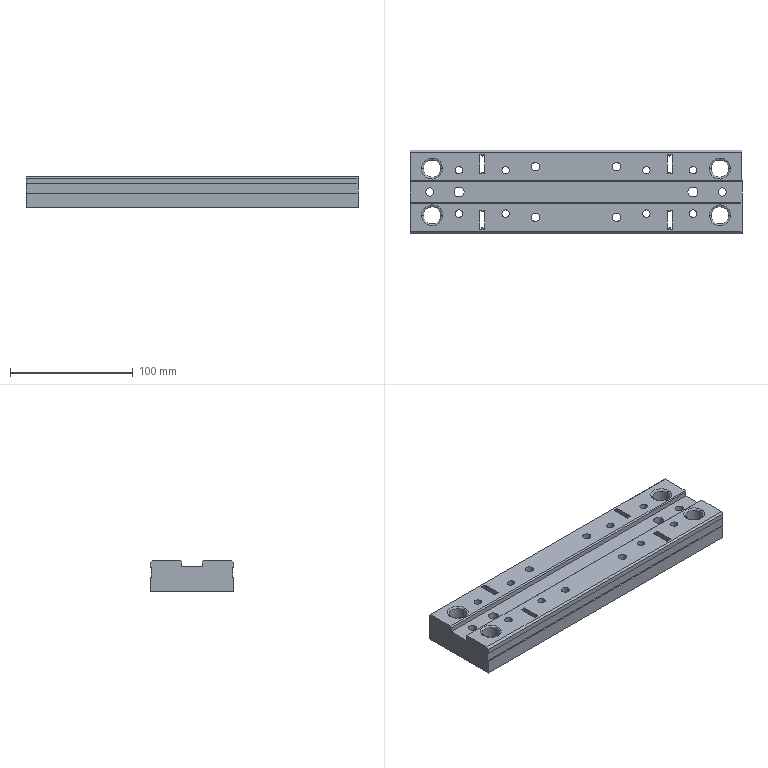Part | STEP file | TAM COI | 1 solid | 262 faces | box 270 x 68 x 25 mm | volume 392735 mm3 | plane 102 | cylinder 96 | cone 56 | spline 8 | commonest cylinder face diameters 0.43 x32 8 x20 5.98 x16 6.647 x12 1.57 x8 13.99 x8